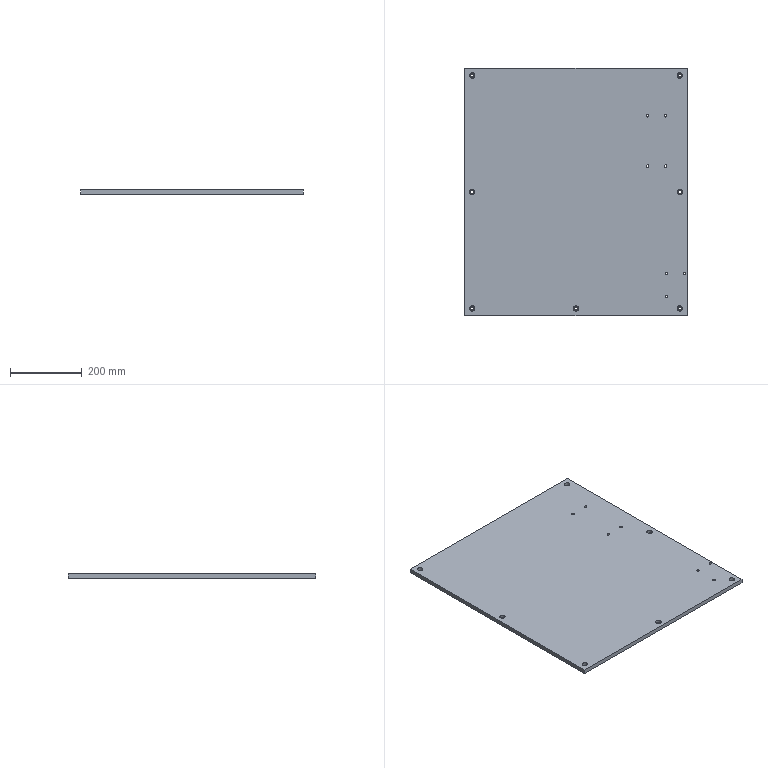Part | STEP file | X77-03003 | 1 solid | 55 faces | box 620 x 690 x 12 mm | volume 5118080 mm3 | cylinder 42 | plane 13 | commonest cylinder face diameters 6.8 x14 9 x14 15 x14